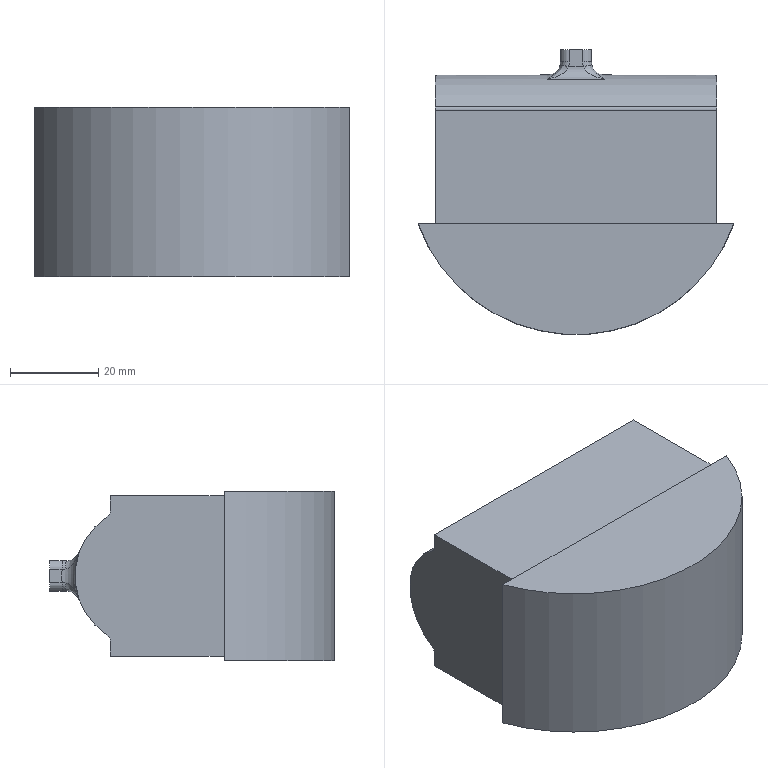CAM job | NX | 3-axis milling | part box 71.627 x 64.667 x 38.42 mm | stock box 71.627 x 64.667 x 38.42 mm
Tools:
number,name,description,diameter,corner_radius,flute_length,length,flutes
0,D10,Milling Tool-5 Parameters,10.0,0.0,50.0,75.0,2
0,B4,Milling Tool-Ball Mill,4.0,2.0,50.0,75.0,2
Operations:
program,operation,operation_type,tool,method,geometry_group,spindle_rpm,surface_speed,feed_per_tooth,feed_cut,feed_plunge,cut_length_mm,path_length_mm,cut_time_min,machine_time_min
NC_PROGRAM,CAVITY_MILL,CavityMilling,D10,METHOD,WORKPIECE,2992.0,282.0,0.4178,2500.0,50.0,27236.256,28432.736,11.389,11.592
NC_PROGRAM,ZLEVEL_PROFILE,ZLevelMilling,B4,METHOD,MCS_MILL,3000.0,282.0,0.4167,2500.0,80.0,2615.765,2641.108,1.047,1.05
NC_PROGRAM,CONTOUR_AREA,SurfaceContour,B4,METHOD,MCS_MILL,3000.0,282.0,0.4167,2500.0,500.0,24522.113,24737.836,9.825,9.847